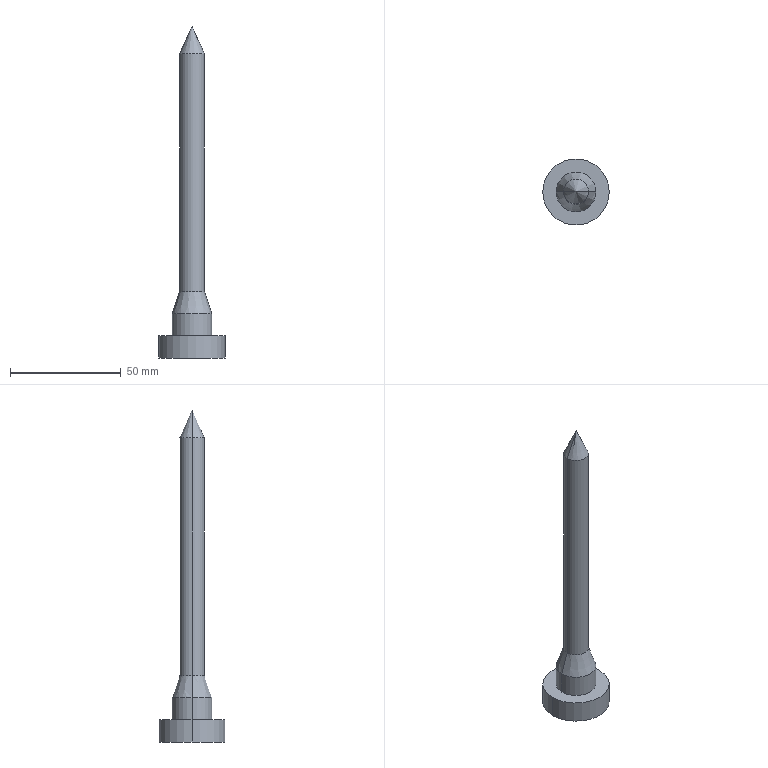Part | SolidWorks | features Extrusion 1, Revolution 1 | 1 solid | 12 faces | box 30 x 30 x 150 mm | volume 22263 mm3 | cylinder 6 | cone 4 | plane 2 | commonest cylinder face diameters 11.172 x2 18 x2 30 x2
STEP:
#1=CARTESIAN_POINT('',(0.,0.,150.));
#2=VERTEX_POINT('',#1);
#3=CARTESIAN_POINT('',(-5.586,0.,137.527));
#4=VERTEX_POINT('',#3);
#5=CARTESIAN_POINT('',(0.,0.,150.));
#6=DIRECTION('',(-0.4087,0.,-0.9127));
#7=VECTOR('',#6,1000.);
#8=LINE('',#5,#7);
#9=EDGE_CURVE('',#2,#4,#8,.T.);
#10=ORIENTED_EDGE('',*,*,#9,.F.);
#11=CARTESIAN_POINT('',(5.586,0.,137.527));
#12=VERTEX_POINT('',#11);
#13=CARTESIAN_POINT('',(0.,0.,150.));
#14=DIRECTION('',(0.4087,0.,-0.9127));
#15=VECTOR('',#14,1000.);
#16=LINE('',#13,#15);
#17=EDGE_CURVE('',#2,#12,#16,.T.);
#18=ORIENTED_EDGE('',*,*,#17,.T.);
#19=CARTESIAN_POINT('',(0.,0.,137.527));
#20=DIRECTION('',(0.,0.,-1.));
#21=DIRECTION('',(-1.,0.,0.));
#22=AXIS2_PLACEMENT_3D('',#19,#20,#21);
#23=CIRCLE('',#22,5.586);
#24=EDGE_CURVE('',#4,#12,#23,.T.);
#25=ORIENTED_EDGE('',*,*,#24,.F.);
#26=EDGE_LOOP('',(#10,#18,#25));
#27=FACE_OUTER_BOUND('',#26,.T.);
#28=CARTESIAN_POINT('',(0.,0.,-850.));
#29=DIRECTION('',(0.,0.,-1.));
#30=DIRECTION('',(-1.,0.,0.));
#31=AXIS2_PLACEMENT_3D('',#28,#29,#30);
#32=CONICAL_SURFACE('',#31,447.835,0.4211);
#33=ADVANCED_FACE('',(#27),#32,.T.);
#34=ORIENTED_EDGE('',*,*,#24,.T.);
#35=CARTESIAN_POINT('',(5.586,0.,30.));
#36=VERTEX_POINT('',#35);
#37=CARTESIAN_POINT('',(5.586,0.,-14.23));
#38=DIRECTION('',(0.,0.,-1.));
#39=VECTOR('',#38,1000.);
#40=LINE('',#37,#39);
#41=EDGE_CURVE('',#12,#36,#40,.T.);
#42=ORIENTED_EDGE('',*,*,#41,.T.);
#43=CARTESIAN_POINT('',(-5.586,0.,30.));
#44=VERTEX_POINT('',#43);
#45=CARTESIAN_POINT('',(0.,0.,30.));
#46=DIRECTION('',(0.,0.,-1.));
#47=DIRECTION('',(-1.,0.,0.));
#48=AXIS2_PLACEMENT_3D('',#45,#46,#47);
#49=CIRCLE('',#48,5.586);
#50=EDGE_CURVE('',#44,#36,#49,.T.);
#51=ORIENTED_EDGE('',*,*,#50,.F.);
#52=CARTESIAN_POINT('',(-5.586,0.,-14.23));
#53=DIRECTION('',(0.,0.,-1.));
#54=VECTOR('',#53,1000.);
#55=LINE('',#52,#54);
#56=EDGE_CURVE('',#4,#44,#55,.T.);
#57=ORIENTED_EDGE('',*,*,#56,.F.);
#58=EDGE_LOOP('',(#34,#42,#51,#57));
#59=FACE_OUTER_BOUND('',#58,.T.);
#60=CARTESIAN_POINT('',(0.,0.,-14.23));
#61=DIRECTION('',(0.,0.,-1.));
#62=DIRECTION('',(-1.,0.,0.));
#63=AXIS2_PLACEMENT_3D('',#60,#61,#62);
#64=CYLINDRICAL_SURFACE('',#63,5.586);
#65=ADVANCED_FACE('',(#59),#64,.T.);
#66=ORIENTED_EDGE('',*,*,#50,.T.);
#67=CARTESIAN_POINT('',(9.,0.,20.));
#68=VERTEX_POINT('',#67);
#69=CARTESIAN_POINT('',(5.586,0.,30.));
#70=DIRECTION('',(0.3231,0.,-0.9464));
#71=VECTOR('',#70,1000.);
#72=LINE('',#69,#71);
#73=EDGE_CURVE('',#36,#68,#72,.T.);
#74=ORIENTED_EDGE('',*,*,#73,.T.);
#75=CARTESIAN_POINT('',(-9.,0.,20.));
#76=VERTEX_POINT('',#75);
#77=CARTESIAN_POINT('',(0.,0.,20.));
#78=DIRECTION('',(0.,0.,-1.));
#79=DIRECTION('',(-1.,0.,0.));
#80=AXIS2_PLACEMENT_3D('',#77,#78,#79);
#81=CIRCLE('',#80,9.);
#82=EDGE_CURVE('',#76,#68,#81,.T.);
#83=ORIENTED_EDGE('',*,*,#82,.F.);
#84=CARTESIAN_POINT('',(-5.586,0.,30.));
#85=DIRECTION('',(-0.3231,0.,-0.9464));
#86=VECTOR('',#85,1000.);
#87=LINE('',#84,#86);
#88=EDGE_CURVE('',#44,#76,#87,.T.);
#89=ORIENTED_EDGE('',*,*,#88,.F.);
#90=EDGE_LOOP('',(#66,#74,#83,#89));
#91=FACE_OUTER_BOUND('',#90,.T.);
#92=CARTESIAN_POINT('',(0.,0.,30.));
#93=DIRECTION('',(0.,0.,-1.));
#94=DIRECTION('',(-1.,0.,0.));
#95=AXIS2_PLACEMENT_3D('',#92,#93,#94);
#96=CONICAL_SURFACE('',#95,5.586,0.329);
#97=ADVANCED_FACE('',(#91),#96,.T.);
#98=ORIENTED_EDGE('',*,*,#82,.T.);
#99=CARTESIAN_POINT('',(9.,0.,10.));
#100=VERTEX_POINT('',#99);
#101=CARTESIAN_POINT('',(9.,0.,-14.23));
#102=DIRECTION('',(0.,0.,-1.));
#103=VECTOR('',#102,1000.);
#104=LINE('',#101,#103);
#105=EDGE_CURVE('',#68,#100,#104,.T.);
#106=ORIENTED_EDGE('',*,*,#105,.T.);
#107=CARTESIAN_POINT('',(-9.,0.,10.));
#108=VERTEX_POINT('',#107);
#109=CARTESIAN_POINT('',(0.,0.,10.));
#110=DIRECTION('',(0.,0.,-1.));
#111=DIRECTION('',(-1.,0.,0.));
#112=AXIS2_PLACEMENT_3D('',#109,#110,#111);
#113=CIRCLE('',#112,9.);
#114=EDGE_CURVE('',#108,#100,#113,.T.);
#115=ORIENTED_EDGE('',*,*,#114,.F.);
#116=CARTESIAN_POINT('',(-9.,0.,-14.23));
#117=DIRECTION('',(0.,0.,-1.));
#118=VECTOR('',#117,1000.);
#119=LINE('',#116,#118);
#120=EDGE_CURVE('',#76,#108,#119,.T.);
#121=ORIENTED_EDGE('',*,*,#120,.F.);
#122=EDGE_LOOP('',(#98,#106,#115,#121));
#123=FACE_OUTER_BOUND('',#122,.T.);
#124=CARTESIAN_POINT('',(0.,0.,-14.23));
#125=DIRECTION('',(0.,0.,-1.));
#126=DIRECTION('',(-1.,0.,0.));
#127=AXIS2_PLACEMENT_3D('',#124,#125,#126);
#128=CYLINDRICAL_SURFACE('',#127,9.);
#129=ADVANCED_FACE('',(#123),#128,.T.);
#130=CARTESIAN_POINT('',(15.,0.,10.));
#131=VERTEX_POINT('',#130);
#132=CARTESIAN_POINT('',(-15.,0.,10.));
#133=VERTEX_POINT('',#132);
#134=CARTESIAN_POINT('',(0.,0.,10.));
#135=DIRECTION('',(0.,0.,1.));
#136=DIRECTION('',(1.,0.,0.));
#137=AXIS2_PLACEMENT_3D('',#134,#135,#136);
#138=CIRCLE('',#137,15.);
#139=EDGE_CURVE('',#131,#133,#138,.T.);
#140=ORIENTED_EDGE('',*,*,#139,.F.);
#141=CARTESIAN_POINT('',(15.,0.,0.));
#142=VERTEX_POINT('',#141);
#143=CARTESIAN_POINT('',(15.,0.,10.));
#144=DIRECTION('',(0.,0.,-1.));
#145=VECTOR('',#144,1000.);
#146=LINE('',#143,#145);
#147=EDGE_CURVE('',#131,#142,#146,.T.);
#148=ORIENTED_EDGE('',*,*,#147,.T.);
#149=CARTESIAN_POINT('',(-15.,0.,0.));
#150=VERTEX_POINT('',#149);
#151=CARTESIAN_POINT('',(0.,0.,0.));
#152=DIRECTION('',(0.,0.,1.));
#153=DIRECTION('',(1.,0.,0.));
#154=AXIS2_PLACEMENT_3D('',#151,#152,#153);
#155=CIRCLE('',#154,15.);
#156=EDGE_CURVE('',#142,#150,#155,.T.);
#157=ORIENTED_EDGE('',*,*,#156,.T.);
#158=CARTESIAN_POINT('',(-15.,0.,10.));
#159=DIRECTION('',(0.,0.,-1.));
#160=VECTOR('',#159,1000.);
#161=LINE('',#158,#160);
#162=EDGE_CURVE('',#133,#150,#161,.T.);
#163=ORIENTED_EDGE('',*,*,#162,.F.);
#164=EDGE_LOOP('',(#140,#148,#157,#163));
#165=FACE_OUTER_BOUND('',#164,.T.);
#166=CARTESIAN_POINT('',(0.,0.,10.));
#167=DIRECTION('',(0.,0.,-1.));
#168=DIRECTION('',(-1.,0.,0.));
#169=AXIS2_PLACEMENT_3D('',#166,#167,#168);
#170=CYLINDRICAL_SURFACE('',#169,15.);
#171=ADVANCED_FACE('',(#165),#170,.T.);
#172=CARTESIAN_POINT('',(0.,0.,10.));
#173=DIRECTION('',(0.,0.,1.));
#174=DIRECTION('',(1.,0.,0.));
#175=AXIS2_PLACEMENT_3D('',#172,#173,#174);
#176=CIRCLE('',#175,15.);
#177=EDGE_CURVE('',#133,#131,#176,.T.);
#178=ORIENTED_EDGE('',*,*,#177,.T.);
#179=ORIENTED_EDGE('',*,*,#139,.T.);
#180=EDGE_LOOP('',(#178,#179));
#181=FACE_OUTER_BOUND('',#180,.T.);
#182=ORIENTED_EDGE('',*,*,#114,.T.);
#183=CARTESIAN_POINT('',(0.,0.,10.));
#184=DIRECTION('',(0.,0.,-1.));
#185=DIRECTION('',(-1.,0.,0.));
#186=AXIS2_PLACEMENT_3D('',#183,#184,#185);
#187=CIRCLE('',#186,9.);
#188=EDGE_CURVE('',#100,#108,#187,.T.);
#189=ORIENTED_EDGE('',*,*,#188,.T.);
#190=EDGE_LOOP('',(#182,#189));
#191=FACE_BOUND('',#190,.T.);
#192=CARTESIAN_POINT('',(0.,0.,10.));
#193=DIRECTION('',(0.,0.,1.));
#194=DIRECTION('',(1.,0.,0.));
#195=AXIS2_PLACEMENT_3D('',#192,#193,#194);
#196=PLANE('',#195);
#197=ADVANCED_FACE('',(#181,#191),#196,.T.);
#198=ORIENTED_EDGE('',*,*,#147,.F.);
#199=ORIENTED_EDGE('',*,*,#177,.F.);
#200=ORIENTED_EDGE('',*,*,#162,.T.);
#201=CARTESIAN_POINT('',(0.,0.,0.));
#202=DIRECTION('',(0.,0.,1.));
#203=DIRECTION('',(1.,0.,0.));
#204=AXIS2_PLACEMENT_3D('',#201,#202,#203);
#205=CIRCLE('',#204,15.);
#206=EDGE_CURVE('',#150,#142,#205,.T.);
#207=ORIENTED_EDGE('',*,*,#206,.T.);
#208=EDGE_LOOP('',(#198,#199,#200,#207));
#209=FACE_OUTER_BOUND('',#208,.T.);
#210=CARTESIAN_POINT('',(0.,0.,10.));
#211=DIRECTION('',(0.,0.,-1.));
#212=DIRECTION('',(-1.,0.,0.));
#213=AXIS2_PLACEMENT_3D('',#210,#211,#212);
#214=CYLINDRICAL_SURFACE('',#213,15.);
#215=ADVANCED_FACE('',(#209),#214,.T.);
#216=ORIENTED_EDGE('',*,*,#206,.F.);
#217=ORIENTED_EDGE('',*,*,#156,.F.);
#218=EDGE_LOOP('',(#216,#217));
#219=FACE_OUTER_BOUND('',#218,.T.);
#220=CARTESIAN_POINT('',(0.,0.,0.));
#221=DIRECTION('',(0.,0.,1.));
#222=DIRECTION('',(1.,0.,0.));
#223=AXIS2_PLACEMENT_3D('',#220,#221,#222);
#224=PLANE('',#223);
#225=ADVANCED_FACE('',(#219),#224,.F.);
#226=ORIENTED_EDGE('',*,*,#105,.F.);
#227=CARTESIAN_POINT('',(0.,0.,20.));
#228=DIRECTION('',(0.,0.,-1.));
#229=DIRECTION('',(-1.,0.,0.));
#230=AXIS2_PLACEMENT_3D('',#227,#228,#229);
#231=CIRCLE('',#230,9.);
#232=EDGE_CURVE('',#68,#76,#231,.T.);
#233=ORIENTED_EDGE('',*,*,#232,.T.);
#234=ORIENTED_EDGE('',*,*,#120,.T.);
#235=ORIENTED_EDGE('',*,*,#188,.F.);
#236=EDGE_LOOP('',(#226,#233,#234,#235));
#237=FACE_OUTER_BOUND('',#236,.T.);
#238=CARTESIAN_POINT('',(0.,0.,-14.23));
#239=DIRECTION('',(0.,0.,-1.));
#240=DIRECTION('',(-1.,0.,0.));
#241=AXIS2_PLACEMENT_3D('',#238,#239,#240);
#242=CYLINDRICAL_SURFACE('',#241,9.);
#243=ADVANCED_FACE('',(#237),#242,.T.);
#244=ORIENTED_EDGE('',*,*,#73,.F.);
#245=CARTESIAN_POINT('',(0.,0.,30.));
#246=DIRECTION('',(0.,0.,-1.));
#247=DIRECTION('',(-1.,0.,0.));
#248=AXIS2_PLACEMENT_3D('',#245,#246,#247);
#249=CIRCLE('',#248,5.586);
#250=EDGE_CURVE('',#36,#44,#249,.T.);
#251=ORIENTED_EDGE('',*,*,#250,.T.);
#252=ORIENTED_EDGE('',*,*,#88,.T.);
#253=ORIENTED_EDGE('',*,*,#232,.F.);
#254=EDGE_LOOP('',(#244,#251,#252,#253));
#255=FACE_OUTER_BOUND('',#254,.T.);
#256=CARTESIAN_POINT('',(0.,0.,30.));
#257=DIRECTION('',(0.,0.,-1.));
#258=DIRECTION('',(-1.,0.,0.));
#259=AXIS2_PLACEMENT_3D('',#256,#257,#258);
#260=CONICAL_SURFACE('',#259,5.586,0.329);
#261=ADVANCED_FACE('',(#255),#260,.T.);
#262=ORIENTED_EDGE('',*,*,#41,.F.);
#263=CARTESIAN_POINT('',(0.,0.,137.527));
#264=DIRECTION('',(0.,0.,-1.));
#265=DIRECTION('',(-1.,0.,0.));
#266=AXIS2_PLACEMENT_3D('',#263,#264,#265);
#267=CIRCLE('',#266,5.586);
#268=EDGE_CURVE('',#12,#4,#267,.T.);
#269=ORIENTED_EDGE('',*,*,#268,.T.);
#270=ORIENTED_EDGE('',*,*,#56,.T.);
#271=ORIENTED_EDGE('',*,*,#250,.F.);
#272=EDGE_LOOP('',(#262,#269,#270,#271));
#273=FACE_OUTER_BOUND('',#272,.T.);
#274=CARTESIAN_POINT('',(0.,0.,-14.23));
#275=DIRECTION('',(0.,0.,-1.));
#276=DIRECTION('',(-1.,0.,0.));
#277=AXIS2_PLACEMENT_3D('',#274,#275,#276);
#278=CYLINDRICAL_SURFACE('',#277,5.586);
#279=ADVANCED_FACE('',(#273),#278,.T.);
#280=ORIENTED_EDGE('',*,*,#17,.F.);
#281=ORIENTED_EDGE('',*,*,#9,.T.);
#282=ORIENTED_EDGE('',*,*,#268,.F.);
#283=EDGE_LOOP('',(#280,#281,#282));
#284=FACE_OUTER_BOUND('',#283,.T.);
#285=CARTESIAN_POINT('',(0.,0.,-850.));
#286=DIRECTION('',(0.,0.,-1.));
#287=DIRECTION('',(-1.,0.,0.));
#288=AXIS2_PLACEMENT_3D('',#285,#286,#287);
#289=CONICAL_SURFACE('',#288,447.835,0.4211);
#290=ADVANCED_FACE('',(#284),#289,.T.);
#291=CLOSED_SHELL('',(#33,#65,#97,#129,#171,#197,#215,#225,#243,#261,#279,#290));
#292=MANIFOLD_SOLID_BREP('',#291);
#293=CARTESIAN_POINT('',(0.,0.,0.));
#294=DIRECTION('',(0.,0.,1.));
#295=DIRECTION('',(1.,0.,0.));
#296=AXIS2_PLACEMENT_3D('',#293,#294,#295);
#297=(LENGTH_UNIT()NAMED_UNIT(*)SI_UNIT(.MILLI.,.METRE.));
#298=UNCERTAINTY_MEASURE_WITH_UNIT(LENGTH_MEASURE(0.00001),#297,'','');
#299=(NAMED_UNIT(*)PLANE_ANGLE_UNIT()SI_UNIT($,.RADIAN.));
#300=(NAMED_UNIT(*)SI_UNIT($,.STERADIAN.)SOLID_ANGLE_UNIT());
#301=(GEOMETRIC_REPRESENTATION_CONTEXT(3)GLOBAL_UNCERTAINTY_ASSIGNED_CONTEXT((#298))GLOBAL_UNIT_ASSIGNED_CONTEXT((#297,#299,#300))REPRESENTATION_CONTEXT('',''));
#302=ADVANCED_BREP_SHAPE_REPRESENTATION('',(#292,#296),#301);